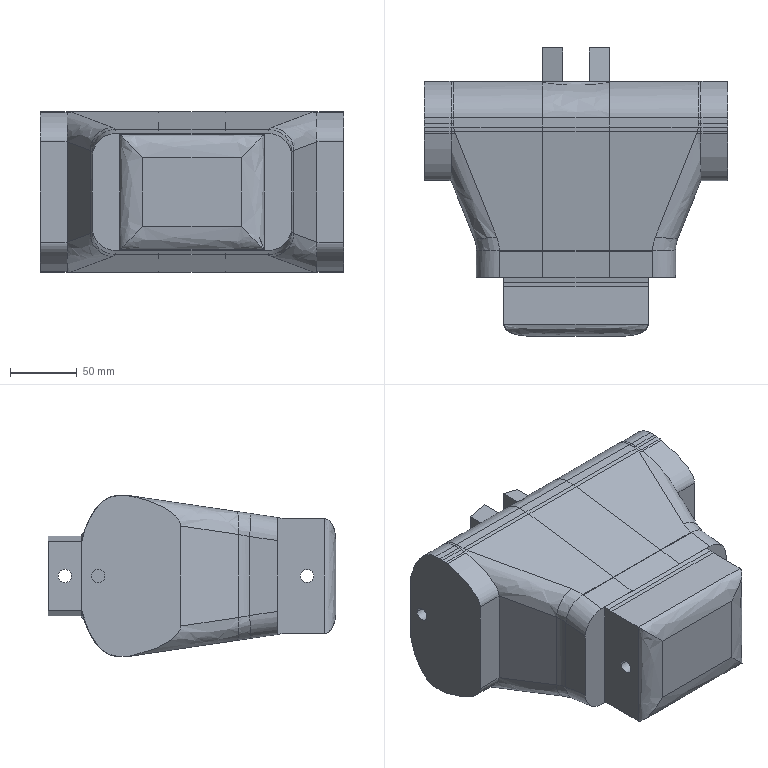Part | SolidWorks | features ICE 19, Fillet 4, MoveCopyBody 4, Revolution 2, Scale 2, Split 1 | 6 solids | 172 faces | box 227 x 215.464 x 120.276 mm | volume 3397637 mm3 | plane 78 | spline 76 | cylinder 18 | commonest cylinder face diameters 10.1 x8 10 x6 34.365 x4